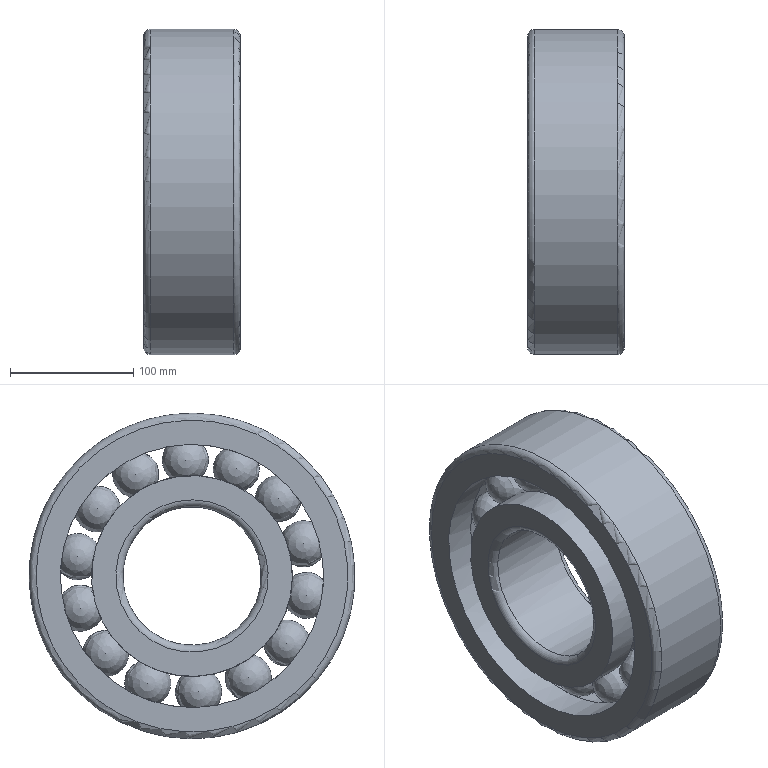Part | NX | features 29.SLDPRT 2, Delete Body 1, LINKED_BODY 1, SCALE 1 | 1 solid | 56 faces | box 78.75 x 264.375 x 264.375 mm | volume 2601399 mm3 | torus 32 | sphere 14 | cylinder 6 | plane 4 | commonest cylinder face diameters 163.125 x2 213.75 x2 112.5 x1 264.375 x1